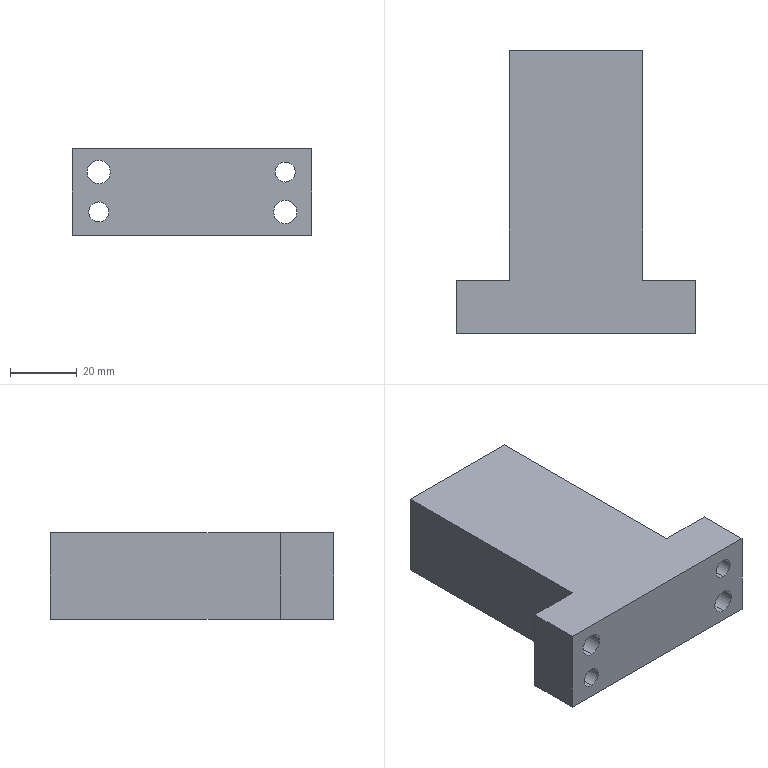Part | SolidWorks | features ICE 4, Extrusion 1 | 1 solid | 36 faces | box 72 x 85 x 26 mm | volume 97502 mm3 | cylinder 20 | plane 16 | commonest cylinder face diameters 5 x8 6 x4 7 x4 12 x4
STEP:
#1=CARTESIAN_POINT('',(-3.,70.,2.5));
#2=VERTEX_POINT('',#1);
#3=CARTESIAN_POINT('',(-3.,70.,7.5));
#4=VERTEX_POINT('',#3);
#5=CARTESIAN_POINT('',(-3.,70.,5.));
#6=DIRECTION('',(0.,1.,0.));
#7=DIRECTION('',(0.,0.,1.));
#8=AXIS2_PLACEMENT_3D('',#5,#6,#7);
#9=CIRCLE('',#8,2.5);
#10=EDGE_CURVE('',#2,#4,#9,.T.);
#11=ORIENTED_EDGE('',*,*,#10,.F.);
#12=CARTESIAN_POINT('',(-3.,85.,2.5));
#13=VERTEX_POINT('',#12);
#14=CARTESIAN_POINT('',(-3.,70.,2.5));
#15=DIRECTION('',(0.,1.,0.));
#16=VECTOR('',#15,1000.);
#17=LINE('',#14,#16);
#18=EDGE_CURVE('',#2,#13,#17,.T.);
#19=ORIENTED_EDGE('',*,*,#18,.T.);
#20=CARTESIAN_POINT('',(-3.,85.,7.5));
#21=VERTEX_POINT('',#20);
#22=CARTESIAN_POINT('',(-3.,85.,5.));
#23=DIRECTION('',(0.,1.,0.));
#24=DIRECTION('',(0.,0.,1.));
#25=AXIS2_PLACEMENT_3D('',#22,#23,#24);
#26=CIRCLE('',#25,2.5);
#27=EDGE_CURVE('',#13,#21,#26,.T.);
#28=ORIENTED_EDGE('',*,*,#27,.T.);
#29=CARTESIAN_POINT('',(-3.,70.,7.5));
#30=DIRECTION('',(0.,1.,0.));
#31=VECTOR('',#30,1000.);
#32=LINE('',#29,#31);
#33=EDGE_CURVE('',#4,#21,#32,.T.);
#34=ORIENTED_EDGE('',*,*,#33,.F.);
#35=EDGE_LOOP('',(#11,#19,#28,#34));
#36=FACE_OUTER_BOUND('',#35,.T.);
#37=CARTESIAN_POINT('',(-3.,70.,5.));
#38=DIRECTION('',(0.,1.,0.));
#39=DIRECTION('',(0.,0.,1.));
#40=AXIS2_PLACEMENT_3D('',#37,#38,#39);
#41=CYLINDRICAL_SURFACE('',#40,2.5);
#42=ADVANCED_FACE('',(#36),#41,.F.);
#43=CARTESIAN_POINT('',(11.,70.,2.5));
#44=VERTEX_POINT('',#43);
#45=CARTESIAN_POINT('',(11.,70.,7.5));
#46=VERTEX_POINT('',#45);
#47=CARTESIAN_POINT('',(11.,70.,5.));
#48=DIRECTION('',(0.,1.,0.));
#49=DIRECTION('',(0.,0.,1.));
#50=AXIS2_PLACEMENT_3D('',#47,#48,#49);
#51=CIRCLE('',#50,2.5);
#52=EDGE_CURVE('',#44,#46,#51,.T.);
#53=ORIENTED_EDGE('',*,*,#52,.F.);
#54=CARTESIAN_POINT('',(11.,85.,2.5));
#55=VERTEX_POINT('',#54);
#56=CARTESIAN_POINT('',(11.,70.,2.5));
#57=DIRECTION('',(0.,1.,0.));
#58=VECTOR('',#57,1000.);
#59=LINE('',#56,#58);
#60=EDGE_CURVE('',#44,#55,#59,.T.);
#61=ORIENTED_EDGE('',*,*,#60,.T.);
#62=CARTESIAN_POINT('',(11.,85.,7.5));
#63=VERTEX_POINT('',#62);
#64=CARTESIAN_POINT('',(11.,85.,5.));
#65=DIRECTION('',(0.,1.,0.));
#66=DIRECTION('',(0.,0.,1.));
#67=AXIS2_PLACEMENT_3D('',#64,#65,#66);
#68=CIRCLE('',#67,2.5);
#69=EDGE_CURVE('',#55,#63,#68,.T.);
#70=ORIENTED_EDGE('',*,*,#69,.T.);
#71=CARTESIAN_POINT('',(11.,70.,7.5));
#72=DIRECTION('',(0.,1.,0.));
#73=VECTOR('',#72,1000.);
#74=LINE('',#71,#73);
#75=EDGE_CURVE('',#46,#63,#74,.T.);
#76=ORIENTED_EDGE('',*,*,#75,.F.);
#77=EDGE_LOOP('',(#53,#61,#70,#76));
#78=FACE_OUTER_BOUND('',#77,.T.);
#79=CARTESIAN_POINT('',(11.,70.,5.));
#80=DIRECTION('',(0.,1.,0.));
#81=DIRECTION('',(0.,0.,1.));
#82=AXIS2_PLACEMENT_3D('',#79,#80,#81);
#83=CYLINDRICAL_SURFACE('',#82,2.5);
#84=ADVANCED_FACE('',(#78),#83,.F.);
#85=CARTESIAN_POINT('',(11.,70.,-7.5));
#86=VERTEX_POINT('',#85);
#87=CARTESIAN_POINT('',(11.,70.,-2.5));
#88=VERTEX_POINT('',#87);
#89=CARTESIAN_POINT('',(11.,70.,-5.));
#90=DIRECTION('',(0.,1.,0.));
#91=DIRECTION('',(0.,0.,1.));
#92=AXIS2_PLACEMENT_3D('',#89,#90,#91);
#93=CIRCLE('',#92,2.5);
#94=EDGE_CURVE('',#86,#88,#93,.T.);
#95=ORIENTED_EDGE('',*,*,#94,.F.);
#96=CARTESIAN_POINT('',(11.,85.,-7.5));
#97=VERTEX_POINT('',#96);
#98=CARTESIAN_POINT('',(11.,70.,-7.5));
#99=DIRECTION('',(0.,1.,0.));
#100=VECTOR('',#99,1000.);
#101=LINE('',#98,#100);
#102=EDGE_CURVE('',#86,#97,#101,.T.);
#103=ORIENTED_EDGE('',*,*,#102,.T.);
#104=CARTESIAN_POINT('',(11.,85.,-2.5));
#105=VERTEX_POINT('',#104);
#106=CARTESIAN_POINT('',(11.,85.,-5.));
#107=DIRECTION('',(0.,1.,0.));
#108=DIRECTION('',(0.,0.,1.));
#109=AXIS2_PLACEMENT_3D('',#106,#107,#108);
#110=CIRCLE('',#109,2.5);
#111=EDGE_CURVE('',#97,#105,#110,.T.);
#112=ORIENTED_EDGE('',*,*,#111,.T.);
#113=CARTESIAN_POINT('',(11.,70.,-2.5));
#114=DIRECTION('',(0.,1.,0.));
#115=VECTOR('',#114,1000.);
#116=LINE('',#113,#115);
#117=EDGE_CURVE('',#88,#105,#116,.T.);
#118=ORIENTED_EDGE('',*,*,#117,.F.);
#119=EDGE_LOOP('',(#95,#103,#112,#118));
#120=FACE_OUTER_BOUND('',#119,.T.);
#121=CARTESIAN_POINT('',(11.,70.,-5.));
#122=DIRECTION('',(0.,1.,0.));
#123=DIRECTION('',(0.,0.,1.));
#124=AXIS2_PLACEMENT_3D('',#121,#122,#123);
#125=CYLINDRICAL_SURFACE('',#124,2.5);
#126=ADVANCED_FACE('',(#120),#125,.F.);
#127=CARTESIAN_POINT('',(-3.,70.,-7.5));
#128=VERTEX_POINT('',#127);
#129=CARTESIAN_POINT('',(-3.,70.,-2.5));
#130=VERTEX_POINT('',#129);
#131=CARTESIAN_POINT('',(-3.,70.,-5.));
#132=DIRECTION('',(0.,1.,0.));
#133=DIRECTION('',(0.,0.,1.));
#134=AXIS2_PLACEMENT_3D('',#131,#132,#133);
#135=CIRCLE('',#134,2.5);
#136=EDGE_CURVE('',#128,#130,#135,.T.);
#137=ORIENTED_EDGE('',*,*,#136,.F.);
#138=CARTESIAN_POINT('',(-3.,85.,-7.5));
#139=VERTEX_POINT('',#138);
#140=CARTESIAN_POINT('',(-3.,70.,-7.5));
#141=DIRECTION('',(0.,1.,0.));
#142=VECTOR('',#141,1000.);
#143=LINE('',#140,#142);
#144=EDGE_CURVE('',#128,#139,#143,.T.);
#145=ORIENTED_EDGE('',*,*,#144,.T.);
#146=CARTESIAN_POINT('',(-3.,85.,-2.5));
#147=VERTEX_POINT('',#146);
#148=CARTESIAN_POINT('',(-3.,85.,-5.));
#149=DIRECTION('',(0.,1.,0.));
#150=DIRECTION('',(0.,0.,1.));
#151=AXIS2_PLACEMENT_3D('',#148,#149,#150);
#152=CIRCLE('',#151,2.5);
#153=EDGE_CURVE('',#139,#147,#152,.T.);
#154=ORIENTED_EDGE('',*,*,#153,.T.);
#155=CARTESIAN_POINT('',(-3.,70.,-2.5));
#156=DIRECTION('',(0.,1.,0.));
#157=VECTOR('',#156,1000.);
#158=LINE('',#155,#157);
#159=EDGE_CURVE('',#130,#147,#158,.T.);
#160=ORIENTED_EDGE('',*,*,#159,.F.);
#161=EDGE_LOOP('',(#137,#145,#154,#160));
#162=FACE_OUTER_BOUND('',#161,.T.);
#163=CARTESIAN_POINT('',(-3.,70.,-5.));
#164=DIRECTION('',(0.,1.,0.));
#165=DIRECTION('',(0.,0.,1.));
#166=AXIS2_PLACEMENT_3D('',#163,#164,#165);
#167=CYLINDRICAL_SURFACE('',#166,2.5);
#168=ADVANCED_FACE('',(#162),#167,.F.);
#169=CARTESIAN_POINT('',(-28.,10.,0.));
#170=VERTEX_POINT('',#169);
#171=CARTESIAN_POINT('',(-28.,10.,12.));
#172=VERTEX_POINT('',#171);
#173=CARTESIAN_POINT('',(-28.,10.,6.));
#174=DIRECTION('',(0.,1.,0.));
#175=DIRECTION('',(0.,0.,1.));
#176=AXIS2_PLACEMENT_3D('',#173,#174,#175);
#177=CIRCLE('',#176,6.);
#178=EDGE_CURVE('',#170,#172,#177,.T.);
#179=ORIENTED_EDGE('',*,*,#178,.F.);
#180=CARTESIAN_POINT('',(-28.,16.,0.));
#181=VERTEX_POINT('',#180);
#182=CARTESIAN_POINT('',(-28.,10.,0.));
#183=DIRECTION('',(0.,1.,0.));
#184=VECTOR('',#183,1000.);
#185=LINE('',#182,#184);
#186=EDGE_CURVE('',#170,#181,#185,.T.);
#187=ORIENTED_EDGE('',*,*,#186,.T.);
#188=CARTESIAN_POINT('',(-28.,16.,12.));
#189=VERTEX_POINT('',#188);
#190=CARTESIAN_POINT('',(-28.,16.,6.));
#191=DIRECTION('',(0.,1.,0.));
#192=DIRECTION('',(0.,0.,1.));
#193=AXIS2_PLACEMENT_3D('',#190,#191,#192);
#194=CIRCLE('',#193,6.);
#195=EDGE_CURVE('',#181,#189,#194,.T.);
#196=ORIENTED_EDGE('',*,*,#195,.T.);
#197=CARTESIAN_POINT('',(-28.,10.,12.));
#198=DIRECTION('',(0.,1.,0.));
#199=VECTOR('',#198,1000.);
#200=LINE('',#197,#199);
#201=EDGE_CURVE('',#172,#189,#200,.T.);
#202=ORIENTED_EDGE('',*,*,#201,.F.);
#203=EDGE_LOOP('',(#179,#187,#196,#202));
#204=FACE_OUTER_BOUND('',#203,.T.);
#205=CARTESIAN_POINT('',(-28.,10.,6.));
#206=DIRECTION('',(0.,1.,0.));
#207=DIRECTION('',(0.,0.,1.));
#208=AXIS2_PLACEMENT_3D('',#205,#206,#207);
#209=CYLINDRICAL_SURFACE('',#208,6.);
#210=ADVANCED_FACE('',(#204),#209,.F.);
#211=CARTESIAN_POINT('',(28.,10.,-12.));
#212=VERTEX_POINT('',#211);
#213=CARTESIAN_POINT('',(28.,10.,0.));
#214=VERTEX_POINT('',#213);
#215=CARTESIAN_POINT('',(28.,10.,-6.));
#216=DIRECTION('',(0.,1.,0.));
#217=DIRECTION('',(0.,0.,1.));
#218=AXIS2_PLACEMENT_3D('',#215,#216,#217);
#219=CIRCLE('',#218,6.);
#220=EDGE_CURVE('',#212,#214,#219,.T.);
#221=ORIENTED_EDGE('',*,*,#220,.F.);
#222=CARTESIAN_POINT('',(28.,16.,-12.));
#223=VERTEX_POINT('',#222);
#224=CARTESIAN_POINT('',(28.,10.,-12.));
#225=DIRECTION('',(0.,1.,0.));
#226=VECTOR('',#225,1000.);
#227=LINE('',#224,#226);
#228=EDGE_CURVE('',#212,#223,#227,.T.);
#229=ORIENTED_EDGE('',*,*,#228,.T.);
#230=CARTESIAN_POINT('',(28.,16.,0.));
#231=VERTEX_POINT('',#230);
#232=CARTESIAN_POINT('',(28.,16.,-6.));
#233=DIRECTION('',(0.,1.,0.));
#234=DIRECTION('',(0.,0.,1.));
#235=AXIS2_PLACEMENT_3D('',#232,#233,#234);
#236=CIRCLE('',#235,6.);
#237=EDGE_CURVE('',#223,#231,#236,.T.);
#238=ORIENTED_EDGE('',*,*,#237,.T.);
#239=CARTESIAN_POINT('',(28.,10.,0.));
#240=DIRECTION('',(0.,1.,0.));
#241=VECTOR('',#240,1000.);
#242=LINE('',#239,#241);
#243=EDGE_CURVE('',#214,#231,#242,.T.);
#244=ORIENTED_EDGE('',*,*,#243,.F.);
#245=EDGE_LOOP('',(#221,#229,#238,#244));
#246=FACE_OUTER_BOUND('',#245,.T.);
#247=CARTESIAN_POINT('',(28.,10.,-6.));
#248=DIRECTION('',(0.,1.,0.));
#249=DIRECTION('',(0.,0.,1.));
#250=AXIS2_PLACEMENT_3D('',#247,#248,#249);
#251=CYLINDRICAL_SURFACE('',#250,6.);
#252=ADVANCED_FACE('',(#246),#251,.F.);
#253=CARTESIAN_POINT('',(-28.,0.,-9.));
#254=VERTEX_POINT('',#253);
#255=CARTESIAN_POINT('',(-28.,0.,-3.));
#256=VERTEX_POINT('',#255);
#257=CARTESIAN_POINT('',(-28.,0.,-6.));
#258=DIRECTION('',(0.,1.,0.));
#259=DIRECTION('',(0.,0.,1.));
#260=AXIS2_PLACEMENT_3D('',#257,#258,#259);
#261=CIRCLE('',#260,3.);
#262=EDGE_CURVE('',#254,#256,#261,.T.);
#263=ORIENTED_EDGE('',*,*,#262,.F.);
#264=CARTESIAN_POINT('',(-28.,16.,-9.));
#265=VERTEX_POINT('',#264);
#266=CARTESIAN_POINT('',(-28.,-80.5,-9.));
#267=DIRECTION('',(0.,1.,0.));
#268=VECTOR('',#267,1000.);
#269=LINE('',#266,#268);
#270=EDGE_CURVE('',#254,#265,#269,.T.);
#271=ORIENTED_EDGE('',*,*,#270,.T.);
#272=CARTESIAN_POINT('',(-28.,16.,-3.));
#273=VERTEX_POINT('',#272);
#274=CARTESIAN_POINT('',(-28.,16.,-6.));
#275=DIRECTION('',(0.,1.,0.));
#276=DIRECTION('',(0.,0.,1.));
#277=AXIS2_PLACEMENT_3D('',#274,#275,#276);
#278=CIRCLE('',#277,3.);
#279=EDGE_CURVE('',#265,#273,#278,.T.);
#280=ORIENTED_EDGE('',*,*,#279,.T.);
#281=CARTESIAN_POINT('',(-28.,-80.5,-3.));
#282=DIRECTION('',(0.,1.,0.));
#283=VECTOR('',#282,1000.);
#284=LINE('',#281,#283);
#285=EDGE_CURVE('',#256,#273,#284,.T.);
#286=ORIENTED_EDGE('',*,*,#285,.F.);
#287=EDGE_LOOP('',(#263,#271,#280,#286));
#288=FACE_OUTER_BOUND('',#287,.T.);
#289=CARTESIAN_POINT('',(-28.,-80.5,-6.));
#290=DIRECTION('',(0.,1.,0.));
#291=DIRECTION('',(0.,0.,1.));
#292=AXIS2_PLACEMENT_3D('',#289,#290,#291);
#293=CYLINDRICAL_SURFACE('',#292,3.);
#294=ADVANCED_FACE('',(#288),#293,.F.);
#295=CARTESIAN_POINT('',(28.,0.,3.));
#296=VERTEX_POINT('',#295);
#297=CARTESIAN_POINT('',(28.,0.,9.));
#298=VERTEX_POINT('',#297);
#299=CARTESIAN_POINT('',(28.,0.,6.));
#300=DIRECTION('',(0.,1.,0.));
#301=DIRECTION('',(0.,0.,1.));
#302=AXIS2_PLACEMENT_3D('',#299,#300,#301);
#303=CIRCLE('',#302,3.);
#304=EDGE_CURVE('',#296,#298,#303,.T.);
#305=ORIENTED_EDGE('',*,*,#304,.F.);
#306=CARTESIAN_POINT('',(28.,16.,3.));
#307=VERTEX_POINT('',#306);
#308=CARTESIAN_POINT('',(28.,-80.5,3.));
#309=DIRECTION('',(0.,1.,0.));
#310=VECTOR('',#309,1000.);
#311=LINE('',#308,#310);
#312=EDGE_CURVE('',#296,#307,#311,.T.);
#313=ORIENTED_EDGE('',*,*,#312,.T.);
#314=CARTESIAN_POINT('',(28.,16.,9.));
#315=VERTEX_POINT('',#314);
#316=CARTESIAN_POINT('',(28.,16.,6.));
#317=DIRECTION('',(0.,1.,0.));
#318=DIRECTION('',(0.,0.,1.));
#319=AXIS2_PLACEMENT_3D('',#316,#317,#318);
#320=CIRCLE('',#319,3.);
#321=EDGE_CURVE('',#307,#315,#320,.T.);
#322=ORIENTED_EDGE('',*,*,#321,.T.);
#323=CARTESIAN_POINT('',(28.,-80.5,9.));
#324=DIRECTION('',(0.,1.,0.));
#325=VECTOR('',#324,1000.);
#326=LINE('',#323,#325);
#327=EDGE_CURVE('',#298,#315,#326,.T.);
#328=ORIENTED_EDGE('',*,*,#327,.F.);
#329=EDGE_LOOP('',(#305,#313,#322,#328));
#330=FACE_OUTER_BOUND('',#329,.T.);
#331=CARTESIAN_POINT('',(28.,-80.5,6.));
#332=DIRECTION('',(0.,1.,0.));
#333=DIRECTION('',(0.,0.,1.));
#334=AXIS2_PLACEMENT_3D('',#331,#332,#333);
#335=CYLINDRICAL_SURFACE('',#334,3.);
#336=ADVANCED_FACE('',(#330),#335,.F.);
#337=CARTESIAN_POINT('',(28.,0.,-9.5));
#338=VERTEX_POINT('',#337);
#339=CARTESIAN_POINT('',(28.,0.,-2.5));
#340=VERTEX_POINT('',#339);
#341=CARTESIAN_POINT('',(28.,0.,-6.));
#342=DIRECTION('',(0.,1.,0.));
#343=DIRECTION('',(0.,0.,1.));
#344=AXIS2_PLACEMENT_3D('',#341,#342,#343);
#345=CIRCLE('',#344,3.5);
#346=EDGE_CURVE('',#338,#340,#345,.T.);
#347=ORIENTED_EDGE('',*,*,#346,.F.);
#348=CARTESIAN_POINT('',(28.,10.,-9.5));
#349=VERTEX_POINT('',#348);
#350=CARTESIAN_POINT('',(28.,-80.5,-9.5));
#351=DIRECTION('',(0.,1.,0.));
#352=VECTOR('',#351,1000.);
#353=LINE('',#350,#352);
#354=EDGE_CURVE('',#338,#349,#353,.T.);
#355=ORIENTED_EDGE('',*,*,#354,.T.);
#356=CARTESIAN_POINT('',(28.,10.,-2.5));
#357=VERTEX_POINT('',#356);
#358=CARTESIAN_POINT('',(28.,10.,-6.));
#359=DIRECTION('',(0.,-1.,0.));
#360=DIRECTION('',(0.,0.,1.));
#361=AXIS2_PLACEMENT_3D('',#358,#359,#360);
#362=CIRCLE('',#361,3.5);
#363=EDGE_CURVE('',#357,#349,#362,.T.);
#364=ORIENTED_EDGE('',*,*,#363,.F.);
#365=CARTESIAN_POINT('',(28.,-80.5,-2.5));
#366=DIRECTION('',(0.,1.,0.));
#367=VECTOR('',#366,1000.);
#368=LINE('',#365,#367);
#369=EDGE_CURVE('',#340,#357,#368,.T.);
#370=ORIENTED_EDGE('',*,*,#369,.F.);
#371=EDGE_LOOP('',(#347,#355,#364,#370));
#372=FACE_OUTER_BOUND('',#371,.T.);
#373=CARTESIAN_POINT('',(28.,-80.5,-6.));
#374=DIRECTION('',(0.,1.,0.));
#375=DIRECTION('',(0.,0.,1.));
#376=AXIS2_PLACEMENT_3D('',#373,#374,#375);
#377=CYLINDRICAL_SURFACE('',#376,3.5);
#378=ADVANCED_FACE('',(#372),#377,.F.);
#379=CARTESIAN_POINT('',(-28.,0.,2.5));
#380=VERTEX_POINT('',#379);
#381=CARTESIAN_POINT('',(-28.,0.,9.5));
#382=VERTEX_POINT('',#381);
#383=CARTESIAN_POINT('',(-28.,0.,6.));
#384=DIRECTION('',(0.,1.,0.));
#385=DIRECTION('',(0.,0.,1.));
#386=AXIS2_PLACEMENT_3D('',#383,#384,#385);
#387=CIRCLE('',#386,3.5);
#388=EDGE_CURVE('',#380,#382,#387,.T.);
#389=ORIENTED_EDGE('',*,*,#388,.F.);
#390=CARTESIAN_POINT('',(-28.,10.,2.5));
#391=VERTEX_POINT('',#390);
#392=CARTESIAN_POINT('',(-28.,-80.5,2.5));
#393=DIRECTION('',(0.,1.,0.));
#394=VECTOR('',#393,1000.);
#395=LINE('',#392,#394);
#396=EDGE_CURVE('',#380,#391,#395,.T.);
#397=ORIENTED_EDGE('',*,*,#396,.T.);
#398=CARTESIAN_POINT('',(-28.,10.,9.5));
#399=VERTEX_POINT('',#398);
#400=CARTESIAN_POINT('',(-28.,10.,6.));
#401=DIRECTION('',(0.,-1.,0.));
#402=DIRECTION('',(0.,0.,1.));
#403=AXIS2_PLACEMENT_3D('',#400,#401,#402);
#404=CIRCLE('',#403,3.5);
#405=EDGE_CURVE('',#399,#391,#404,.T.);
#406=ORIENTED_EDGE('',*,*,#405,.F.);
#407=CARTESIAN_POINT('',(-28.,-80.5,9.5));
#408=DIRECTION('',(0.,1.,0.));
#409=VECTOR('',#408,1000.);
#410=LINE('',#407,#409);
#411=EDGE_CURVE('',#382,#399,#410,.T.);
#412=ORIENTED_EDGE('',*,*,#411,.F.);
#413=EDGE_LOOP('',(#389,#397,#406,#412));
#414=FACE_OUTER_BOUND('',#413,.T.);
#415=CARTESIAN_POINT('',(-28.,-80.5,6.));
#416=DIRECTION('',(0.,1.,0.));
#417=DIRECTION('',(0.,0.,1.));
#418=AXIS2_PLACEMENT_3D('',#415,#416,#417);
#419=CYLINDRICAL_SURFACE('',#418,3.5);
#420=ADVANCED_FACE('',(#414),#419,.F.);
#421=ORIENTED_EDGE('',*,*,#396,.F.);
#422=CARTESIAN_POINT('',(-28.,0.,6.));
#423=DIRECTION('',(0.,1.,0.));
#424=DIRECTION('',(0.,0.,1.));
#425=AXIS2_PLACEMENT_3D('',#422,#423,#424);
#426=CIRCLE('',#425,3.5);
#427=EDGE_CURVE('',#382,#380,#426,.T.);
#428=ORIENTED_EDGE('',*,*,#427,.F.);
#429=ORIENTED_EDGE('',*,*,#411,.T.);
#430=CARTESIAN_POINT('',(-28.,10.,6.));
#431=DIRECTION('',(0.,-1.,0.));
#432=DIRECTION('',(0.,0.,1.));
#433=AXIS2_PLACEMENT_3D('',#430,#431,#432);
#434=CIRCLE('',#433,3.5);
#435=EDGE_CURVE('',#391,#399,#434,.T.);
#436=ORIENTED_EDGE('',*,*,#435,.F.);
#437=EDGE_LOOP('',(#421,#428,#429,#436));
#438=FACE_OUTER_BOUND('',#437,.T.);
#439=CARTESIAN_POINT('',(-28.,-80.5,6.));
#440=DIRECTION('',(0.,1.,0.));
#441=DIRECTION('',(0.,0.,1.));
#442=AXIS2_PLACEMENT_3D('',#439,#440,#441);
#443=CYLINDRICAL_SURFACE('',#442,3.5);
#444=ADVANCED_FACE('',(#438),#443,.F.);
#445=ORIENTED_EDGE('',*,*,#354,.F.);
#446=CARTESIAN_POINT('',(28.,0.,-6.));
#447=DIRECTION('',(0.,1.,0.));
#448=DIRECTION('',(0.,0.,1.));
#449=AXIS2_PLACEMENT_3D('',#446,#447,#448);
#450=CIRCLE('',#449,3.5);
#451=EDGE_CURVE('',#340,#338,#450,.T.);
#452=ORIENTED_EDGE('',*,*,#451,.F.);
#453=ORIENTED_EDGE('',*,*,#369,.T.);
#454=CARTESIAN_POINT('',(28.,10.,-6.));
#455=DIRECTION('',(0.,-1.,0.));
#456=DIRECTION('',(0.,0.,1.));
#457=AXIS2_PLACEMENT_3D('',#454,#455,#456);
#458=CIRCLE('',#457,3.5);
#459=EDGE_CURVE('',#349,#357,#458,.T.);
#460=ORIENTED_EDGE('',*,*,#459,.F.);
#461=EDGE_LOOP('',(#445,#452,#453,#460));
#462=FACE_OUTER_BOUND('',#461,.T.);
#463=CARTESIAN_POINT('',(28.,-80.5,-6.));
#464=DIRECTION('',(0.,1.,0.));
#465=DIRECTION('',(0.,0.,1.));
#466=AXIS2_PLACEMENT_3D('',#463,#464,#465);
#467=CYLINDRICAL_SURFACE('',#466,3.5);
#468=ADVANCED_FACE('',(#462),#467,.F.);
#469=CARTESIAN_POINT('',(28.,16.,-6.));
#470=DIRECTION('',(0.,1.,0.));
#471=DIRECTION('',(0.,0.,1.));
#472=AXIS2_PLACEMENT_3D('',#469,#470,#471);
#473=CIRCLE('',#472,6.);
#474=EDGE_CURVE('',#231,#223,#473,.T.);
#475=ORIENTED_EDGE('',*,*,#474,.F.);
#476=ORIENTED_EDGE('',*,*,#237,.F.);
#477=EDGE_LOOP('',(#475,#476));
#478=FACE_BOUND('',#477,.T.);
#479=CARTESIAN_POINT('',(28.,16.,6.));
#480=DIRECTION('',(0.,1.,0.));
#481=DIRECTION('',(0.,0.,1.));
#482=AXIS2_PLACEMENT_3D('',#479,#480,#481);
#483=CIRCLE('',#482,3.);
#484=EDGE_CURVE('',#315,#307,#483,.T.);
#485=ORIENTED_EDGE('',*,*,#484,.F.);
#486=ORIENTED_EDGE('',*,*,#321,.F.);
#487=EDGE_LOOP('',(#485,#486));
#488=FACE_BOUND('',#487,.T.);
#489=CARTESIAN_POINT('',(20.,16.,13.));
#490=VERTEX_POINT('',#489);
#491=CARTESIAN_POINT('',(20.,16.,-13.));
#492=VERTEX_POINT('',#491);
#493=CARTESIAN_POINT('',(20.,16.,-13.));
#494=DIRECTION('',(0.,0.,-1.));
#495=VECTOR('',#494,1000.);
#496=LINE('',#493,#495);
#497=EDGE_CURVE('',#490,#492,#496,.T.);
#498=ORIENTED_EDGE('',*,*,#497,.F.);
#499=CARTESIAN_POINT('',(36.,16.,13.));
#500=VERTEX_POINT('',#499);
#501=CARTESIAN_POINT('',(-36.,16.,13.));
#502=DIRECTION('',(1.,0.,0.));
#503=VECTOR('',#502,1000.);
#504=LINE('',#501,#503);
#505=EDGE_CURVE('',#490,#500,#504,.T.);
#506=ORIENTED_EDGE('',*,*,#505,.T.);
#507=CARTESIAN_POINT('',(36.,16.,-13.));
#508=VERTEX_POINT('',#507);
#509=CARTESIAN_POINT('',(36.,16.,-13.));
#510=DIRECTION('',(0.,0.,-1.));
#511=VECTOR('',#510,1000.);
#512=LINE('',#509,#511);
#513=EDGE_CURVE('',#500,#508,#512,.T.);
#514=ORIENTED_EDGE('',*,*,#513,.T.);
#515=CARTESIAN_POINT('',(-36.,16.,-13.));
#516=DIRECTION('',(-1.,0.,0.));
#517=VECTOR('',#516,1000.);
#518=LINE('',#515,#517);
#519=EDGE_CURVE('',#508,#492,#518,.T.);
#520=ORIENTED_EDGE('',*,*,#519,.T.);
#521=EDGE_LOOP('',(#498,#506,#514,#520));
#522=FACE_OUTER_BOUND('',#521,.T.);
#523=CARTESIAN_POINT('',(36.,16.,13.));
#524=DIRECTION('',(0.,1.,0.));
#525=DIRECTION('',(0.,0.,1.));
#526=AXIS2_PLACEMENT_3D('',#523,#524,#525);
#527=PLANE('',#526);
#528=ADVANCED_FACE('',(#478,#488,#522),#527,.T.);
#529=CARTESIAN_POINT('',(36.,0.,13.));
#530=VERTEX_POINT('',#529);
#531=CARTESIAN_POINT('',(36.,0.,-13.));
#532=VERTEX_POINT('',#531);
#533=CARTESIAN_POINT('',(36.,0.,-13.));
#534=DIRECTION('',(0.,0.,-1.));
#535=VECTOR('',#534,1000.);
#536=LINE('',#533,#535);
#537=EDGE_CURVE('',#530,#532,#536,.T.);
#538=ORIENTED_EDGE('',*,*,#537,.T.);
#539=CARTESIAN_POINT('',(36.,16.,-13.));
#540=DIRECTION('',(0.,-1.,0.));
#541=VECTOR('',#540,1000.);
#542=LINE('',#539,#541);
#543=EDGE_CURVE('',#508,#532,#542,.T.);
#544=ORIENTED_EDGE('',*,*,#543,.F.);
#545=ORIENTED_EDGE('',*,*,#513,.F.);
#546=CARTESIAN_POINT('',(36.,16.,13.));
#547=DIRECTION('',(0.,-1.,0.));
#548=VECTOR('',#547,1000.);
#549=LINE('',#546,#548);
#550=EDGE_CURVE('',#500,#530,#549,.T.);
#551=ORIENTED_EDGE('',*,*,#550,.T.);
#552=EDGE_LOOP('',(#538,#544,#545,#551));
#553=FACE_OUTER_BOUND('',#552,.T.);
#554=CARTESIAN_POINT('',(36.,16.,-13.));
#555=DIRECTION('',(-1.,0.,0.));
#556=DIRECTION('',(0.,0.,1.));
#557=AXIS2_PLACEMENT_3D('',#554,#555,#556);
#558=PLANE('',#557);
#559=ADVANCED_FACE('',(#553),#558,.F.);
#560=CARTESIAN_POINT('',(-36.,0.,-13.));
#561=VERTEX_POINT('',#560);
#562=CARTESIAN_POINT('',(-36.,0.,-13.));
#563=DIRECTION('',(-1.,0.,0.));
#564=VECTOR('',#563,1000.);
#565=LINE('',#562,#564);
#566=EDGE_CURVE('',#532,#561,#565,.T.);
#567=ORIENTED_EDGE('',*,*,#566,.T.);
#568=CARTESIAN_POINT('',(-36.,16.,-13.));
#569=VERTEX_POINT('',#568);
#570=CARTESIAN_POINT('',(-36.,16.,-13.));
#571=DIRECTION('',(0.,-1.,0.));
#572=VECTOR('',#571,1000.);
#573=LINE('',#570,#572);
#574=EDGE_CURVE('',#569,#561,#573,.T.);
#575=ORIENTED_EDGE('',*,*,#574,.F.);
#576=CARTESIAN_POINT('',(-20.,16.,-13.));
#577=VERTEX_POINT('',#576);
#578=CARTESIAN_POINT('',(-36.,16.,-13.));
#579=DIRECTION('',(-1.,0.,0.));
#580=VECTOR('',#579,1000.);
#581=LINE('',#578,#580);
#582=EDGE_CURVE('',#577,#569,#581,.T.);
#583=ORIENTED_EDGE('',*,*,#582,.F.);
#584=CARTESIAN_POINT('',(-20.,85.,-13.));
#585=VERTEX_POINT('',#584);
#586=CARTESIAN_POINT('',(-20.,85.,-13.));
#587=DIRECTION('',(0.,-1.,0.));
#588=VECTOR('',#587,1000.);
#589=LINE('',#586,#588);
#590=EDGE_CURVE('',#585,#577,#589,.T.);
#591=ORIENTED_EDGE('',*,*,#590,.F.);
#592=CARTESIAN_POINT('',(20.,85.,-13.));
#593=VERTEX_POINT('',#592);
#594=CARTESIAN_POINT('',(-20.,85.,-13.));
#595=DIRECTION('',(-1.,0.,0.));
#596=VECTOR('',#595,1000.);
#597=LINE('',#594,#596);
#598=EDGE_CURVE('',#593,#585,#597,.T.);
#599=ORIENTED_EDGE('',*,*,#598,.F.);
#600=CARTESIAN_POINT('',(20.,85.,-13.));
#601=DIRECTION('',(0.,-1.,0.));
#602=VECTOR('',#601,1000.);
#603=LINE('',#600,#602);
#604=EDGE_CURVE('',#593,#492,#603,.T.);
#605=ORIENTED_EDGE('',*,*,#604,.T.);
#606=ORIENTED_EDGE('',*,*,#519,.F.);
#607=ORIENTED_EDGE('',*,*,#543,.T.);
#608=EDGE_LOOP('',(#567,#575,#583,#591,#599,#605,#606,#607));
#609=FACE_OUTER_BOUND('',#608,.T.);
#610=CARTESIAN_POINT('',(-36.,16.,-13.));
#611=DIRECTION('',(0.,0.,1.));
#612=DIRECTION('',(1.,0.,0.));
#613=AXIS2_PLACEMENT_3D('',#610,#611,#612);
#614=PLANE('',#613);
#615=ADVANCED_FACE('',(#609),#614,.F.);
#616=CARTESIAN_POINT('',(-36.,0.,13.));
#617=VERTEX_POINT('',#616);
#618=CARTESIAN_POINT('',(-36.,0.,-13.));
#619=DIRECTION('',(0.,0.,1.));
#620=VECTOR('',#619,1000.);
#621=LINE('',#618,#620);
#622=EDGE_CURVE('',#561,#617,#621,.T.);
#623=ORIENTED_EDGE('',*,*,#622,.T.);
#624=CARTESIAN_POINT('',(-36.,16.,13.));
#625=VERTEX_POINT('',#624);
#626=CARTESIAN_POINT('',(-36.,16.,13.));
#627=DIRECTION('',(0.,-1.,0.));
#628=VECTOR('',#627,1000.);
#629=LINE('',#626,#628);
#630=EDGE_CURVE('',#625,#617,#629,.T.);
#631=ORIENTED_EDGE('',*,*,#630,.F.);
#632=CARTESIAN_POINT('',(-36.,16.,-13.));
#633=DIRECTION('',(0.,0.,1.));
#634=VECTOR('',#633,1000.);
#635=LINE('',#632,#634);
#636=EDGE_CURVE('',#569,#625,#635,.T.);
#637=ORIENTED_EDGE('',*,*,#636,.F.);
#638=ORIENTED_EDGE('',*,*,#574,.T.);
#639=EDGE_LOOP('',(#623,#631,#637,#638));
#640=FACE_OUTER_BOUND('',#639,.T.);
#641=CARTESIAN_POINT('',(-36.,16.,-13.));
#642=DIRECTION('',(1.,0.,0.));
#643=DIRECTION('',(0.,0.,-1.));
#644=AXIS2_PLACEMENT_3D('',#641,#642,#643);
#645=PLANE('',#644);
#646=ADVANCED_FACE('',(#640),#645,.F.);
#647=CARTESIAN_POINT('',(-36.,0.,13.));
#648=DIRECTION('',(1.,0.,0.));
#649=VECTOR('',#648,1000.);
#650=LINE('',#647,#649);
#651=EDGE_CURVE('',#617,#530,#650,.T.);
#652=ORIENTED_EDGE('',*,*,#651,.T.);
#653=ORIENTED_EDGE('',*,*,#550,.F.);
#654=ORIENTED_EDGE('',*,*,#505,.F.);
#655=CARTESIAN_POINT('',(20.,85.,13.));
#656=VERTEX_POINT('',#655);
#657=CARTESIAN_POINT('',(20.,85.,13.));
#658=DIRECTION('',(0.,-1.,0.));
#659=VECTOR('',#658,1000.);
#660=LINE('',#657,#659);
#661=EDGE_CURVE('',#656,#490,#660,.T.);
#662=ORIENTED_EDGE('',*,*,#661,.F.);
#663=CARTESIAN_POINT('',(-20.,85.,13.));
#664=VERTEX_POINT('',#663);
#665=CARTESIAN_POINT('',(-20.,85.,13.));
#666=DIRECTION('',(1.,0.,0.));
#667=VECTOR('',#666,1000.);
#668=LINE('',#665,#667);
#669=EDGE_CURVE('',#664,#656,#668,.T.);
#670=ORIENTED_EDGE('',*,*,#669,.F.);
#671=CARTESIAN_POINT('',(-20.,16.,13.));
#672=VERTEX_POINT('',#671);
#673=CARTESIAN_POINT('',(-20.,85.,13.));
#674=DIRECTION('',(0.,-1.,0.));
#675=VECTOR('',#674,1000.);
#676=LINE('',#673,#675);
#677=EDGE_CURVE('',#664,#672,#676,.T.);
#678=ORIENTED_EDGE('',*,*,#677,.T.);
#679=CARTESIAN_POINT('',(-36.,16.,13.));
#680=DIRECTION('',(1.,0.,0.));
#681=VECTOR('',#680,1000.);
#682=LINE('',#679,#681);
#683=EDGE_CURVE('',#625,#672,#682,.T.);
#684=ORIENTED_EDGE('',*,*,#683,.F.);
#685=ORIENTED_EDGE('',*,*,#630,.T.);
#686=EDGE_LOOP('',(#652,#653,#654,#662,#670,#678,#684,#685));
#687=FACE_OUTER_BOUND('',#686,.T.);
#688=CARTESIAN_POINT('',(-36.,16.,13.));
#689=DIRECTION('',(0.,0.,-1.));
#690=DIRECTION('',(-1.,0.,0.));
#691=AXIS2_PLACEMENT_3D('',#688,#689,#690);
#692=PLANE('',#691);
#693=ADVANCED_FACE('',(#687),#692,.F.);
#694=CARTESIAN_POINT('',(-28.,16.,6.));
#695=DIRECTION('',(0.,1.,0.));
#696=DIRECTION('',(0.,0.,1.));
#697=AXIS2_PLACEMENT_3D('',#694,#695,#696);
#698=CIRCLE('',#697,6.);
#699=EDGE_CURVE('',#189,#181,#698,.T.);
#700=ORIENTED_EDGE('',*,*,#699,.F.);
#701=ORIENTED_EDGE('',*,*,#195,.F.);
#702=EDGE_LOOP('',(#700,#701));
#703=FACE_BOUND('',#702,.T.);
#704=CARTESIAN_POINT('',(-28.,16.,-6.));
#705=DIRECTION('',(0.,1.,0.));
#706=DIRECTION('',(0.,0.,1.));
#707=AXIS2_PLACEMENT_3D('',#704,#705,#706);
#708=CIRCLE('',#707,3.);
#709=EDGE_CURVE('',#273,#265,#708,.T.);
#710=ORIENTED_EDGE('',*,*,#709,.F.);
#711=ORIENTED_EDGE('',*,*,#279,.F.);
#712=EDGE_LOOP('',(#710,#711));
#713=FACE_BOUND('',#712,.T.);
#714=CARTESIAN_POINT('',(-20.,16.,-13.));
#715=DIRECTION('',(0.,0.,1.));
#716=VECTOR('',#715,1000.);
#717=LINE('',#714,#716);
#718=EDGE_CURVE('',#577,#672,#717,.T.);
#719=ORIENTED_EDGE('',*,*,#718,.F.);
#720=ORIENTED_EDGE('',*,*,#582,.T.);
#721=ORIENTED_EDGE('',*,*,#636,.T.);
#722=ORIENTED_EDGE('',*,*,#683,.T.);
#723=EDGE_LOOP('',(#719,#720,#721,#722));
#724=FACE_OUTER_BOUND('',#723,.T.);
#725=CARTESIAN_POINT('',(36.,16.,13.));
#726=DIRECTION('',(0.,1.,0.));
#727=DIRECTION('',(0.,0.,1.));
#728=AXIS2_PLACEMENT_3D('',#725,#726,#727);
#729=PLANE('',#728);
#730=ADVANCED_FACE('',(#703,#713,#724),#729,.T.);
#731=CARTESIAN_POINT('',(-28.,0.,-6.));
#732=DIRECTION('',(0.,1.,0.));
#733=DIRECTION('',(0.,0.,1.));
#734=AXIS2_PLACEMENT_3D('',#731,#732,#733);
#735=CIRCLE('',#734,3.);
#736=EDGE_CURVE('',#256,#254,#735,.T.);
#737=ORIENTED_EDGE('',*,*,#736,.T.);
#738=ORIENTED_EDGE('',*,*,#262,.T.);
#739=EDGE_LOOP('',(#737,#738));
#740=FACE_BOUND('',#739,.T.);
#741=ORIENTED_EDGE('',*,*,#427,.T.);
#742=ORIENTED_EDGE('',*,*,#388,.T.);
#743=EDGE_LOOP('',(#741,#742));
#744=FACE_BOUND('',#743,.T.);
#745=CARTESIAN_POINT('',(28.,0.,6.));
#746=DIRECTION('',(0.,1.,0.));
#747=DIRECTION('',(0.,0.,1.));
#748=AXIS2_PLACEMENT_3D('',#745,#746,#747);
#749=CIRCLE('',#748,3.);
#750=EDGE_CURVE('',#298,#296,#749,.T.);
#751=ORIENTED_EDGE('',*,*,#750,.T.);
#752=ORIENTED_EDGE('',*,*,#304,.T.);
#753=EDGE_LOOP('',(#751,#752));
#754=FACE_BOUND('',#753,.T.);
#755=ORIENTED_EDGE('',*,*,#451,.T.);
#756=ORIENTED_EDGE('',*,*,#346,.T.);
#757=EDGE_LOOP('',(#755,#756));
#758=FACE_BOUND('',#757,.T.);
#759=ORIENTED_EDGE('',*,*,#537,.F.);
#760=ORIENTED_EDGE('',*,*,#651,.F.);
#761=ORIENTED_EDGE('',*,*,#622,.F.);
#762=ORIENTED_EDGE('',*,*,#566,.F.);
#763=EDGE_LOOP('',(#759,#760,#761,#762));
#764=FACE_OUTER_BOUND('',#763,.T.);
#765=CARTESIAN_POINT('',(36.,0.,13.));
#766=DIRECTION('',(0.,1.,0.));
#767=DIRECTION('',(0.,0.,1.));
#768=AXIS2_PLACEMENT_3D('',#765,#766,#767);
#769=PLANE('',#768);
#770=ADVANCED_FACE('',(#740,#744,#754,#758,#764),#769,.F.);
#771=ORIENTED_EDGE('',*,*,#497,.T.);
#772=ORIENTED_EDGE('',*,*,#604,.F.);
#773=CARTESIAN_POINT('',(20.,85.,-13.));
#774=DIRECTION('',(0.,0.,-1.));
#775=VECTOR('',#774,1000.);
#776=LINE('',#773,#775);
#777=EDGE_CURVE('',#656,#593,#776,.T.);
#778=ORIENTED_EDGE('',*,*,#777,.F.);
#779=ORIENTED_EDGE('',*,*,#661,.T.);
#780=EDGE_LOOP('',(#771,#772,#778,#779));
#781=FACE_OUTER_BOUND('',#780,.T.);
#782=CARTESIAN_POINT('',(20.,85.,-13.));
#783=DIRECTION('',(-1.,0.,0.));
#784=DIRECTION('',(0.,0.,1.));
#785=AXIS2_PLACEMENT_3D('',#782,#783,#784);
#786=PLANE('',#785);
#787=ADVANCED_FACE('',(#781),#786,.F.);
#788=ORIENTED_EDGE('',*,*,#718,.T.);
#789=ORIENTED_EDGE('',*,*,#677,.F.);
#790=CARTESIAN_POINT('',(-20.,85.,-13.));
#791=DIRECTION('',(0.,0.,1.));
#792=VECTOR('',#791,1000.);
#793=LINE('',#790,#792);
#794=EDGE_CURVE('',#585,#664,#793,.T.);
#795=ORIENTED_EDGE('',*,*,#794,.F.);
#796=ORIENTED_EDGE('',*,*,#590,.T.);
#797=EDGE_LOOP('',(#788,#789,#795,#796));
#798=FACE_OUTER_BOUND('',#797,.T.);
#799=CARTESIAN_POINT('',(-20.,85.,-13.));
#800=DIRECTION('',(1.,0.,0.));
#801=DIRECTION('',(0.,0.,-1.));
#802=AXIS2_PLACEMENT_3D('',#799,#800,#801);
#803=PLANE('',#802);
#804=ADVANCED_FACE('',(#798),#803,.F.);
#805=CARTESIAN_POINT('',(-3.,85.,5.));
#806=DIRECTION('',(0.,1.,0.));
#807=DIRECTION('',(0.,0.,1.));
#808=AXIS2_PLACEMENT_3D('',#805,#806,#807);
#809=CIRCLE('',#808,2.5);
#810=EDGE_CURVE('',#21,#13,#809,.T.);
#811=ORIENTED_EDGE('',*,*,#810,.F.);
#812=ORIENTED_EDGE('',*,*,#27,.F.);
#813=EDGE_LOOP('',(#811,#812));
#814=FACE_BOUND('',#813,.T.);
#815=CARTESIAN_POINT('',(11.,85.,5.));
#816=DIRECTION('',(0.,1.,0.));
#817=DIRECTION('',(0.,0.,1.));
#818=AXIS2_PLACEMENT_3D('',#815,#816,#817);
#819=CIRCLE('',#818,2.5);
#820=EDGE_CURVE('',#63,#55,#819,.T.);
#821=ORIENTED_EDGE('',*,*,#820,.F.);
#822=ORIENTED_EDGE('',*,*,#69,.F.);
#823=EDGE_LOOP('',(#821,#822));
#824=FACE_BOUND('',#823,.T.);
#825=CARTESIAN_POINT('',(11.,85.,-5.));
#826=DIRECTION('',(0.,1.,0.));
#827=DIRECTION('',(0.,0.,1.));
#828=AXIS2_PLACEMENT_3D('',#825,#826,#827);
#829=CIRCLE('',#828,2.5);
#830=EDGE_CURVE('',#105,#97,#829,.T.);
#831=ORIENTED_EDGE('',*,*,#830,.F.);
#832=ORIENTED_EDGE('',*,*,#111,.F.);
#833=EDGE_LOOP('',(#831,#832));
#834=FACE_BOUND('',#833,.T.);
#835=CARTESIAN_POINT('',(-3.,85.,-5.));
#836=DIRECTION('',(0.,1.,0.));
#837=DIRECTION('',(0.,0.,1.));
#838=AXIS2_PLACEMENT_3D('',#835,#836,#837);
#839=CIRCLE('',#838,2.5);
#840=EDGE_CURVE('',#147,#139,#839,.T.);
#841=ORIENTED_EDGE('',*,*,#840,.F.);
#842=ORIENTED_EDGE('',*,*,#153,.F.);
#843=EDGE_LOOP('',(#841,#842));
#844=FACE_BOUND('',#843,.T.);
#845=ORIENTED_EDGE('',*,*,#777,.T.);
#846=ORIENTED_EDGE('',*,*,#598,.T.);
#847=ORIENTED_EDGE('',*,*,#794,.T.);
#848=ORIENTED_EDGE('',*,*,#669,.T.);
#849=EDGE_LOOP('',(#845,#846,#847,#848));
#850=FACE_OUTER_BOUND('',#849,.T.);
#851=CARTESIAN_POINT('',(20.,85.,13.));
#852=DIRECTION('',(0.,1.,0.));
#853=DIRECTION('',(0.,0.,1.));
#854=AXIS2_PLACEMENT_3D('',#851,#852,#853);
#855=PLANE('',#854);
#856=ADVANCED_FACE('',(#814,#824,#834,#844,#850),#855,.T.);
#857=ORIENTED_EDGE('',*,*,#312,.F.);
#858=ORIENTED_EDGE('',*,*,#750,.F.);
#859=ORIENTED_EDGE('',*,*,#327,.T.);
#860=ORIENTED_EDGE('',*,*,#484,.T.);
#861=EDGE_LOOP('',(#857,#858,#859,#860));
#862=FACE_OUTER_BOUND('',#861,.T.);
#863=CARTESIAN_POINT('',(28.,-80.5,6.));
#864=DIRECTION('',(0.,1.,0.));
#865=DIRECTION('',(0.,0.,1.));
#866=AXIS2_PLACEMENT_3D('',#863,#864,#865);
#867=CYLINDRICAL_SURFACE('',#866,3.);
#868=ADVANCED_FACE('',(#862),#867,.F.);
#869=ORIENTED_EDGE('',*,*,#270,.F.);
#870=ORIENTED_EDGE('',*,*,#736,.F.);
#871=ORIENTED_EDGE('',*,*,#285,.T.);
#872=ORIENTED_EDGE('',*,*,#709,.T.);
#873=EDGE_LOOP('',(#869,#870,#871,#872));
#874=FACE_OUTER_BOUND('',#873,.T.);
#875=CARTESIAN_POINT('',(-28.,-80.5,-6.));
#876=DIRECTION('',(0.,1.,0.));
#877=DIRECTION('',(0.,0.,1.));
#878=AXIS2_PLACEMENT_3D('',#875,#876,#877);
#879=CYLINDRICAL_SURFACE('',#878,3.);
#880=ADVANCED_FACE('',(#874),#879,.F.);
#881=CARTESIAN_POINT('',(28.,10.,-6.));
#882=DIRECTION('',(0.,1.,0.));
#883=DIRECTION('',(0.,0.,1.));
#884=AXIS2_PLACEMENT_3D('',#881,#882,#883);
#885=CIRCLE('',#884,6.);
#886=EDGE_CURVE('',#214,#212,#885,.T.);
#887=ORIENTED_EDGE('',*,*,#886,.T.);
#888=ORIENTED_EDGE('',*,*,#220,.T.);
#889=EDGE_LOOP('',(#887,#888));
#890=FACE_OUTER_BOUND('',#889,.T.);
#891=ORIENTED_EDGE('',*,*,#363,.T.);
#892=ORIENTED_EDGE('',*,*,#459,.T.);
#893=EDGE_LOOP('',(#891,#892));
#894=FACE_BOUND('',#893,.T.);
#895=CARTESIAN_POINT('',(28.,10.,-6.));
#896=DIRECTION('',(0.,1.,0.));
#897=DIRECTION('',(0.,0.,1.));
#898=AXIS2_PLACEMENT_3D('',#895,#896,#897);
#899=PLANE('',#898);
#900=ADVANCED_FACE('',(#890,#894),#899,.T.);
#901=ORIENTED_EDGE('',*,*,#228,.F.);
#902=ORIENTED_EDGE('',*,*,#886,.F.);
#903=ORIENTED_EDGE('',*,*,#243,.T.);
#904=ORIENTED_EDGE('',*,*,#474,.T.);
#905=EDGE_LOOP('',(#901,#902,#903,#904));
#906=FACE_OUTER_BOUND('',#905,.T.);
#907=CARTESIAN_POINT('',(28.,10.,-6.));
#908=DIRECTION('',(0.,1.,0.));
#909=DIRECTION('',(0.,0.,1.));
#910=AXIS2_PLACEMENT_3D('',#907,#908,#909);
#911=CYLINDRICAL_SURFACE('',#910,6.);
#912=ADVANCED_FACE('',(#906),#911,.F.);
#913=CARTESIAN_POINT('',(-28.,10.,6.));
#914=DIRECTION('',(0.,1.,0.));
#915=DIRECTION('',(0.,0.,1.));
#916=AXIS2_PLACEMENT_3D('',#913,#914,#915);
#917=CIRCLE('',#916,6.);
#918=EDGE_CURVE('',#172,#170,#917,.T.);
#919=ORIENTED_EDGE('',*,*,#918,.T.);
#920=ORIENTED_EDGE('',*,*,#178,.T.);
#921=EDGE_LOOP('',(#919,#920));
#922=FACE_OUTER_BOUND('',#921,.T.);
#923=ORIENTED_EDGE('',*,*,#405,.T.);
#924=ORIENTED_EDGE('',*,*,#435,.T.);
#925=EDGE_LOOP('',(#923,#924));
#926=FACE_BOUND('',#925,.T.);
#927=CARTESIAN_POINT('',(-28.,10.,6.));
#928=DIRECTION('',(0.,1.,0.));
#929=DIRECTION('',(0.,0.,1.));
#930=AXIS2_PLACEMENT_3D('',#927,#928,#929);
#931=PLANE('',#930);
#932=ADVANCED_FACE('',(#922,#926),#931,.T.);
#933=ORIENTED_EDGE('',*,*,#186,.F.);
#934=ORIENTED_EDGE('',*,*,#918,.F.);
#935=ORIENTED_EDGE('',*,*,#201,.T.);
#936=ORIENTED_EDGE('',*,*,#699,.T.);
#937=EDGE_LOOP('',(#933,#934,#935,#936));
#938=FACE_OUTER_BOUND('',#937,.T.);
#939=CARTESIAN_POINT('',(-28.,10.,6.));
#940=DIRECTION('',(0.,1.,0.));
#941=DIRECTION('',(0.,0.,1.));
#942=AXIS2_PLACEMENT_3D('',#939,#940,#941);
#943=CYLINDRICAL_SURFACE('',#942,6.);
#944=ADVANCED_FACE('',(#938),#943,.F.);
#945=ORIENTED_EDGE('',*,*,#144,.F.);
#946=CARTESIAN_POINT('',(-3.,70.,-5.));
#947=DIRECTION('',(0.,1.,0.));
#948=DIRECTION('',(0.,0.,1.));
#949=AXIS2_PLACEMENT_3D('',#946,#947,#948);
#950=CIRCLE('',#949,2.5);
#951=EDGE_CURVE('',#130,#128,#950,.T.);
#952=ORIENTED_EDGE('',*,*,#951,.F.);
#953=ORIENTED_EDGE('',*,*,#159,.T.);
#954=ORIENTED_EDGE('',*,*,#840,.T.);
#955=EDGE_LOOP('',(#945,#952,#953,#954));
#956=FACE_OUTER_BOUND('',#955,.T.);
#957=CARTESIAN_POINT('',(-3.,70.,-5.));
#958=DIRECTION('',(0.,1.,0.));
#959=DIRECTION('',(0.,0.,1.));
#960=AXIS2_PLACEMENT_3D('',#957,#958,#959);
#961=CYLINDRICAL_SURFACE('',#960,2.5);
#962=ADVANCED_FACE('',(#956),#961,.F.);
#963=ORIENTED_EDGE('',*,*,#951,.T.);
#964=ORIENTED_EDGE('',*,*,#136,.T.);
#965=EDGE_LOOP('',(#963,#964));
#966=FACE_OUTER_BOUND('',#965,.T.);
#967=CARTESIAN_POINT('',(-3.,70.,-5.));
#968=DIRECTION('',(0.,1.,0.));
#969=DIRECTION('',(0.,0.,1.));
#970=AXIS2_PLACEMENT_3D('',#967,#968,#969);
#971=PLANE('',#970);
#972=ADVANCED_FACE('',(#966),#971,.T.);
#973=ORIENTED_EDGE('',*,*,#102,.F.);
#974=CARTESIAN_POINT('',(11.,70.,-5.));
#975=DIRECTION('',(0.,1.,0.));
#976=DIRECTION('',(0.,0.,1.));
#977=AXIS2_PLACEMENT_3D('',#974,#975,#976);
#978=CIRCLE('',#977,2.5);
#979=EDGE_CURVE('',#88,#86,#978,.T.);
#980=ORIENTED_EDGE('',*,*,#979,.F.);
#981=ORIENTED_EDGE('',*,*,#117,.T.);
#982=ORIENTED_EDGE('',*,*,#830,.T.);
#983=EDGE_LOOP('',(#973,#980,#981,#982));
#984=FACE_OUTER_BOUND('',#983,.T.);
#985=CARTESIAN_POINT('',(11.,70.,-5.));
#986=DIRECTION('',(0.,1.,0.));
#987=DIRECTION('',(0.,0.,1.));
#988=AXIS2_PLACEMENT_3D('',#985,#986,#987);
#989=CYLINDRICAL_SURFACE('',#988,2.5);
#990=ADVANCED_FACE('',(#984),#989,.F.);
#991=ORIENTED_EDGE('',*,*,#979,.T.);
#992=ORIENTED_EDGE('',*,*,#94,.T.);
#993=EDGE_LOOP('',(#991,#992));
#994=FACE_OUTER_BOUND('',#993,.T.);
#995=CARTESIAN_POINT('',(11.,70.,-5.));
#996=DIRECTION('',(0.,1.,0.));
#997=DIRECTION('',(0.,0.,1.));
#998=AXIS2_PLACEMENT_3D('',#995,#996,#997);
#999=PLANE('',#998);
#1000=ADVANCED_FACE('',(#994),#999,.T.);
#1001=ORIENTED_EDGE('',*,*,#60,.F.);
#1002=CARTESIAN_POINT('',(11.,70.,5.));
#1003=DIRECTION('',(0.,1.,0.));
#1004=DIRECTION('',(0.,0.,1.));
#1005=AXIS2_PLACEMENT_3D('',#1002,#1003,#1004);
#1006=CIRCLE('',#1005,2.5);
#1007=EDGE_CURVE('',#46,#44,#1006,.T.);
#1008=ORIENTED_EDGE('',*,*,#1007,.F.);
#1009=ORIENTED_EDGE('',*,*,#75,.T.);
#1010=ORIENTED_EDGE('',*,*,#820,.T.);
#1011=EDGE_LOOP('',(#1001,#1008,#1009,#1010));
#1012=FACE_OUTER_BOUND('',#1011,.T.);
#1013=CARTESIAN_POINT('',(11.,70.,5.));
#1014=DIRECTION('',(0.,1.,0.));
#1015=DIRECTION('',(0.,0.,1.));
#1016=AXIS2_PLACEMENT_3D('',#1013,#1014,#1015);
#1017=CYLINDRICAL_SURFACE('',#1016,2.5);
#1018=ADVANCED_FACE('',(#1012),#1017,.F.);
#1019=ORIENTED_EDGE('',*,*,#1007,.T.);
#1020=ORIENTED_EDGE('',*,*,#52,.T.);
#1021=EDGE_LOOP('',(#1019,#1020));
#1022=FACE_OUTER_BOUND('',#1021,.T.);
#1023=CARTESIAN_POINT('',(11.,70.,5.));
#1024=DIRECTION('',(0.,1.,0.));
#1025=DIRECTION('',(0.,0.,1.));
#1026=AXIS2_PLACEMENT_3D('',#1023,#1024,#1025);
#1027=PLANE('',#1026);
#1028=ADVANCED_FACE('',(#1022),#1027,.T.);
#1029=ORIENTED_EDGE('',*,*,#18,.F.);
#1030=CARTESIAN_POINT('',(-3.,70.,5.));
#1031=DIRECTION('',(0.,1.,0.));
#1032=DIRECTION('',(0.,0.,1.));
#1033=AXIS2_PLACEMENT_3D('',#1030,#1031,#1032);
#1034=CIRCLE('',#1033,2.5);
#1035=EDGE_CURVE('',#4,#2,#1034,.T.);
#1036=ORIENTED_EDGE('',*,*,#1035,.F.);
#1037=ORIENTED_EDGE('',*,*,#33,.T.);
#1038=ORIENTED_EDGE('',*,*,#810,.T.);
#1039=EDGE_LOOP('',(#1029,#1036,#1037,#1038));
#1040=FACE_OUTER_BOUND('',#1039,.T.);
#1041=CARTESIAN_POINT('',(-3.,70.,5.));
#1042=DIRECTION('',(0.,1.,0.));
#1043=DIRECTION('',(0.,0.,1.));
#1044=AXIS2_PLACEMENT_3D('',#1041,#1042,#1043);
#1045=CYLINDRICAL_SURFACE('',#1044,2.5);
#1046=ADVANCED_FACE('',(#1040),#1045,.F.);
#1047=ORIENTED_EDGE('',*,*,#1035,.T.);
#1048=ORIENTED_EDGE('',*,*,#10,.T.);
#1049=EDGE_LOOP('',(#1047,#1048));
#1050=FACE_OUTER_BOUND('',#1049,.T.);
#1051=CARTESIAN_POINT('',(-3.,70.,5.));
#1052=DIRECTION('',(0.,1.,0.));
#1053=DIRECTION('',(0.,0.,1.));
#1054=AXIS2_PLACEMENT_3D('',#1051,#1052,#1053);
#1055=PLANE('',#1054);
#1056=ADVANCED_FACE('',(#1050),#1055,.T.);
#1057=CLOSED_SHELL('',(#42,#84,#126,#168,#210,#252,#294,#336,#378,#420,#444,#468,#528,#559,#615,#646,#693,#730,#770,#787,#804,#856,#868,#880,#900,#912,#932,#944,#962,#972,#990,#1000,#1018,#1028,#1046,#1056));
#1058=MANIFOLD_SOLID_BREP('',#1057);
#1059=CARTESIAN_POINT('',(0.,0.,0.));
#1060=DIRECTION('',(0.,0.,1.));
#1061=DIRECTION('',(1.,0.,0.));
#1062=AXIS2_PLACEMENT_3D('',#1059,#1060,#1061);
#1063=(LENGTH_UNIT()NAMED_UNIT(*)SI_UNIT(.MILLI.,.METRE.));
#1064=UNCERTAINTY_MEASURE_WITH_UNIT(LENGTH_MEASURE(0.00001),#1063,'','');
#1065=(NAMED_UNIT(*)PLANE_ANGLE_UNIT()SI_UNIT($,.RADIAN.));
#1066=(NAMED_UNIT(*)SI_UNIT($,.STERADIAN.)SOLID_ANGLE_UNIT());
#1067=(GEOMETRIC_REPRESENTATION_CONTEXT(3)GLOBAL_UNCERTAINTY_ASSIGNED_CONTEXT((#1064))GLOBAL_UNIT_ASSIGNED_CONTEXT((#1063,#1065,#1066))REPRESENTATION_CONTEXT('',''));
#1068=ADVANCED_BREP_SHAPE_REPRESENTATION('',(#1058,#1062),#1067);